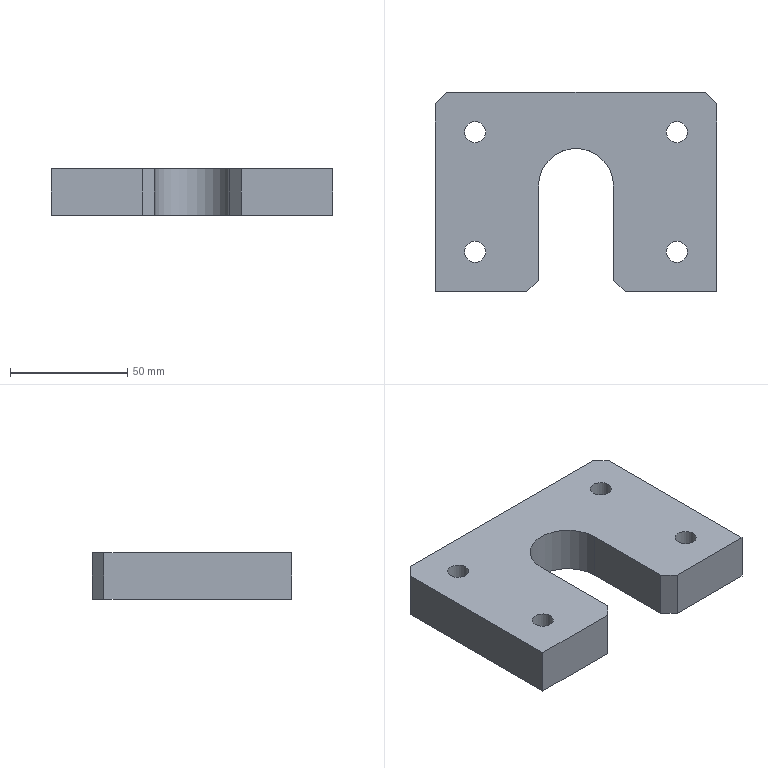Part | STEP file | gslz 2016.10.28-10_id2242_x_t | 1 solid | 26 faces | box 120 x 85 x 20 mm | volume 157455 mm3 | plane 17 | cylinder 9 | commonest cylinder face diameters 9 x4 14 x4 32 x1